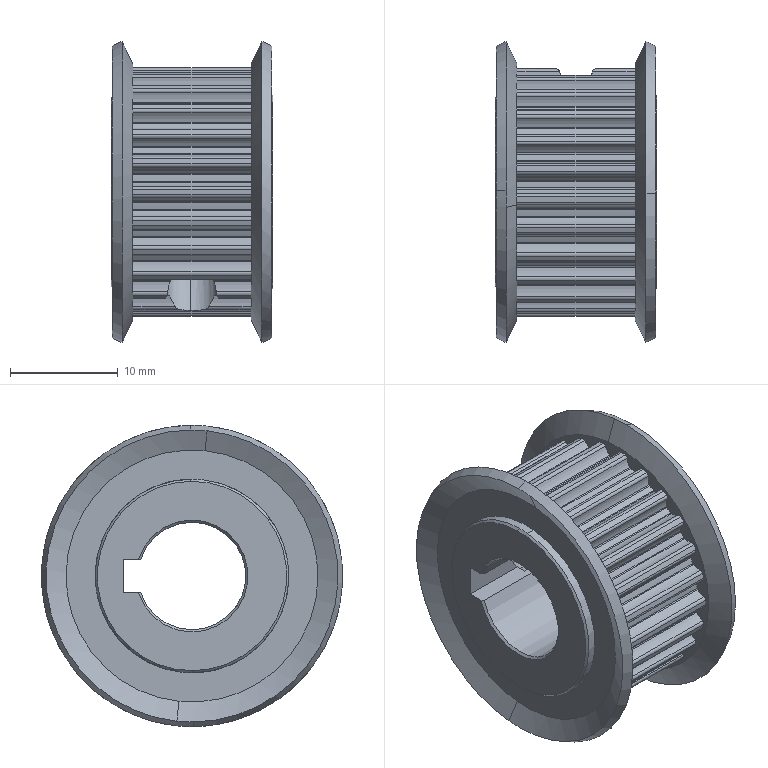Part | STEP file | 11-XMISUMI-HTPA25S3M100-A-N10_HTPA2.PRT11 | 1 solid | 282 faces | box 15 x 28 x 28 mm | volume 4500 mm3 | cylinder 245 | cone 23 | plane 14 | commonest cylinder face diameters 0.3 x58 0.56 x57 3.95 x57 20.89 x28 23.11 x28 3.242 x4